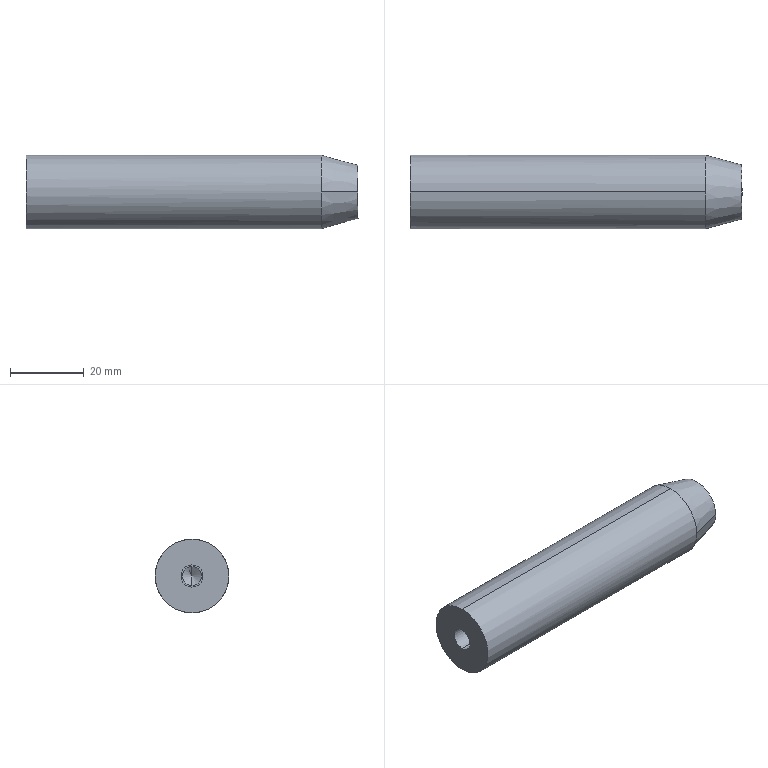Part | STEP file | [01]-15 | 1 solid | 13 faces | box 90 x 20 x 20 mm | volume 27097 mm3 | cylinder 6 | cone 4 | plane 3 | commonest cylinder face diameters 5.1 x2 6 x2 20 x2
STEP:
#1=CARTESIAN_POINT('',(0.,0.,0.));
#2=DIRECTION('',(0.,0.,1.));
#3=DIRECTION('',(1.,0.,0.));
#4=AXIS2_PLACEMENT_3D('',#1,#2,#3);
#5=CARTESIAN_POINT('',(15.,0.,-2.55));
#6=VERTEX_POINT('',#5);
#7=CARTESIAN_POINT('',(15.,0.,2.55));
#8=VERTEX_POINT('',#7);
#9=CARTESIAN_POINT('',(15.,0.,0.));
#10=DIRECTION('',(-1.,0.,0.));
#11=DIRECTION('',(0.,0.,1.));
#12=AXIS2_PLACEMENT_3D('',#9,#10,#11);
#13=CIRCLE('',#12,2.55);
#14=CARTESIAN_POINT('',(15.,0.,0.));
#15=DIRECTION('',(-1.,0.,0.));
#16=DIRECTION('',(0.,0.,1.));
#17=AXIS2_PLACEMENT_3D('',#14,#15,#16);
#18=CONICAL_SURFACE('',#17,2.55,1.03);
#19=CARTESIAN_POINT('',(0.,0.));
#20=DIRECTION('',(1.,0.));
#21=VECTOR('',#20,1.);
#22=LINE('',#19,#21);
#23=(GEOMETRIC_REPRESENTATION_CONTEXT(2)PARAMETRIC_REPRESENTATION_CONTEXT()REPRESENTATION_CONTEXT('',''));
#24=DEFINITIONAL_REPRESENTATION('',(#22),#23);
#25=PCURVE('',#18,#24);
#26=CARTESIAN_POINT('',(0.,0.,0.));
#27=DIRECTION('',(-1.,0.,0.));
#28=DIRECTION('',(0.,0.,1.));
#29=AXIS2_PLACEMENT_3D('',#26,#27,#28);
#30=CYLINDRICAL_SURFACE('',#29,2.55);
#31=CARTESIAN_POINT('',(0.,-15.));
#32=DIRECTION('',(1.,0.));
#33=VECTOR('',#32,1.);
#34=LINE('',#31,#33);
#35=(GEOMETRIC_REPRESENTATION_CONTEXT(2)PARAMETRIC_REPRESENTATION_CONTEXT()REPRESENTATION_CONTEXT('',''));
#36=DEFINITIONAL_REPRESENTATION('',(#34),#35);
#37=PCURVE('',#30,#36);
#38=SURFACE_CURVE('',#13,(#25,#37),.PCURVE_S1.);
#39=EDGE_CURVE('',#6,#8,#38,.T.);
#40=ORIENTED_EDGE('',*,*,#39,.F.);
#41=CARTESIAN_POINT('',(16.532,0.,0.));
#42=VERTEX_POINT('',#41);
#43=CARTESIAN_POINT('',(15.,0.,-2.55));
#44=DIRECTION('',(-0.515,0.,-0.8572));
#45=VECTOR('',#44,1.);
#46=LINE('',#43,#45);
#47=CARTESIAN_POINT('',(3.142,0.));
#48=DIRECTION('',(0.,1.));
#49=VECTOR('',#48,1.);
#50=LINE('',#47,#49);
#51=(GEOMETRIC_REPRESENTATION_CONTEXT(2)PARAMETRIC_REPRESENTATION_CONTEXT()REPRESENTATION_CONTEXT('',''));
#52=DEFINITIONAL_REPRESENTATION('',(#50),#51);
#53=PCURVE('',#18,#52);
#54=CARTESIAN_POINT('',(15.,0.,0.));
#55=DIRECTION('',(-1.,0.,0.));
#56=DIRECTION('',(0.,0.,1.));
#57=AXIS2_PLACEMENT_3D('',#54,#55,#56);
#58=CONICAL_SURFACE('',#57,2.55,1.03);
#59=CARTESIAN_POINT('',(3.142,0.));
#60=DIRECTION('',(0.,1.));
#61=VECTOR('',#60,1.);
#62=LINE('',#59,#61);
#63=(GEOMETRIC_REPRESENTATION_CONTEXT(2)PARAMETRIC_REPRESENTATION_CONTEXT()REPRESENTATION_CONTEXT('',''));
#64=DEFINITIONAL_REPRESENTATION('',(#62),#63);
#65=PCURVE('',#58,#64);
#66=SURFACE_CURVE('',#46,(#53,#65),.PCURVE_S1.);
#67=EDGE_CURVE('',#42,#6,#66,.T.);
#68=ORIENTED_EDGE('',*,*,#67,.F.);
#69=CARTESIAN_POINT('',(15.,0.,2.55));
#70=DIRECTION('',(-0.515,0.,0.8572));
#71=VECTOR('',#70,1.);
#72=LINE('',#69,#71);
#73=CARTESIAN_POINT('',(6.283,0.));
#74=DIRECTION('',(0.,1.));
#75=VECTOR('',#74,1.);
#76=LINE('',#73,#75);
#77=(GEOMETRIC_REPRESENTATION_CONTEXT(2)PARAMETRIC_REPRESENTATION_CONTEXT()REPRESENTATION_CONTEXT('',''));
#78=DEFINITIONAL_REPRESENTATION('',(#76),#77);
#79=PCURVE('',#18,#78);
#80=CARTESIAN_POINT('',(0.,0.));
#81=DIRECTION('',(0.,1.));
#82=VECTOR('',#81,1.);
#83=LINE('',#80,#82);
#84=(GEOMETRIC_REPRESENTATION_CONTEXT(2)PARAMETRIC_REPRESENTATION_CONTEXT()REPRESENTATION_CONTEXT('',''));
#85=DEFINITIONAL_REPRESENTATION('',(#83),#84);
#86=PCURVE('',#58,#85);
#87=SURFACE_CURVE('',#72,(#79,#86),.PCURVE_S1.);
#88=EDGE_CURVE('',#42,#8,#87,.T.);
#89=ORIENTED_EDGE('',*,*,#88,.T.);
#90=EDGE_LOOP('',(#40,#68,#89));
#91=FACE_BOUND('',#90,.F.);
#92=ADVANCED_FACE('',(#91),#18,.F.);
#93=CARTESIAN_POINT('',(12.,0.,2.55));
#94=VERTEX_POINT('',#93);
#95=CARTESIAN_POINT('',(0.,0.,2.55));
#96=DIRECTION('',(-1.,0.,0.));
#97=VECTOR('',#96,1.);
#98=LINE('',#95,#97);
#99=CARTESIAN_POINT('',(6.283,0.));
#100=DIRECTION('',(0.,1.));
#101=VECTOR('',#100,1.);
#102=LINE('',#99,#101);
#103=(GEOMETRIC_REPRESENTATION_CONTEXT(2)PARAMETRIC_REPRESENTATION_CONTEXT()REPRESENTATION_CONTEXT('',''));
#104=DEFINITIONAL_REPRESENTATION('',(#102),#103);
#105=PCURVE('',#30,#104);
#106=CARTESIAN_POINT('',(0.,0.,0.));
#107=DIRECTION('',(-1.,0.,0.));
#108=DIRECTION('',(0.,0.,1.));
#109=AXIS2_PLACEMENT_3D('',#106,#107,#108);
#110=CYLINDRICAL_SURFACE('',#109,2.55);
#111=CARTESIAN_POINT('',(0.,0.));
#112=DIRECTION('',(0.,1.));
#113=VECTOR('',#112,1.);
#114=LINE('',#111,#113);
#115=(GEOMETRIC_REPRESENTATION_CONTEXT(2)PARAMETRIC_REPRESENTATION_CONTEXT()REPRESENTATION_CONTEXT('',''));
#116=DEFINITIONAL_REPRESENTATION('',(#114),#115);
#117=PCURVE('',#110,#116);
#118=SURFACE_CURVE('',#98,(#105,#117),.PCURVE_S1.);
#119=EDGE_CURVE('',#8,#94,#118,.T.);
#120=ORIENTED_EDGE('',*,*,#119,.T.);
#121=CARTESIAN_POINT('',(12.,0.,-2.55));
#122=VERTEX_POINT('',#121);
#123=CARTESIAN_POINT('',(12.,0.,0.));
#124=DIRECTION('',(-1.,0.,0.));
#125=DIRECTION('',(0.,0.,1.));
#126=AXIS2_PLACEMENT_3D('',#123,#124,#125);
#127=CIRCLE('',#126,2.55);
#128=CARTESIAN_POINT('',(0.,-12.));
#129=DIRECTION('',(1.,0.));
#130=VECTOR('',#129,1.);
#131=LINE('',#128,#130);
#132=(GEOMETRIC_REPRESENTATION_CONTEXT(2)PARAMETRIC_REPRESENTATION_CONTEXT()REPRESENTATION_CONTEXT('',''));
#133=DEFINITIONAL_REPRESENTATION('',(#131),#132);
#134=PCURVE('',#30,#133);
#135=CARTESIAN_POINT('',(12.,0.,-3.));
#136=DIRECTION('',(1.,0.,0.));
#137=DIRECTION('',(0.,0.,-1.));
#138=AXIS2_PLACEMENT_3D('',#135,#136,#137);
#139=PLANE('',#138);
#140=CARTESIAN_POINT('',(-5.55,0.));
#141=CARTESIAN_POINT('',(-5.55,4.417));
#142=CARTESIAN_POINT('',(-1.725,2.208));
#143=CARTESIAN_POINT('',(2.1,0.));
#144=CARTESIAN_POINT('',(-1.725,-2.208));
#145=CARTESIAN_POINT('',(-5.55,-4.417));
#146=CARTESIAN_POINT('',(-5.55,0.));
#147=(BOUNDED_CURVE()B_SPLINE_CURVE(2,(#140,#141,#142,#143,#144,#145,#146),.UNSPECIFIED.,.T.,.F.)B_SPLINE_CURVE_WITH_KNOTS((1,2,2,2,2,1),(-2.094,0.,2.094,4.189,6.283,8.378),.UNSPECIFIED.)CURVE()GEOMETRIC_REPRESENTATION_ITEM()RATIONAL_B_SPLINE_CURVE((1.,0.5,1.,0.5,1.,0.5,1.))REPRESENTATION_ITEM(''));
#148=(GEOMETRIC_REPRESENTATION_CONTEXT(2)PARAMETRIC_REPRESENTATION_CONTEXT()REPRESENTATION_CONTEXT('',''));
#149=DEFINITIONAL_REPRESENTATION('',(#147),#148);
#150=PCURVE('',#139,#149);
#151=SURFACE_CURVE('',#127,(#134,#150),.PCURVE_S1.);
#152=EDGE_CURVE('',#122,#94,#151,.T.);
#153=ORIENTED_EDGE('',*,*,#152,.F.);
#154=CARTESIAN_POINT('',(0.,0.,-2.55));
#155=DIRECTION('',(-1.,0.,0.));
#156=VECTOR('',#155,1.);
#157=LINE('',#154,#156);
#158=CARTESIAN_POINT('',(3.142,0.));
#159=DIRECTION('',(0.,1.));
#160=VECTOR('',#159,1.);
#161=LINE('',#158,#160);
#162=(GEOMETRIC_REPRESENTATION_CONTEXT(2)PARAMETRIC_REPRESENTATION_CONTEXT()REPRESENTATION_CONTEXT('',''));
#163=DEFINITIONAL_REPRESENTATION('',(#161),#162);
#164=PCURVE('',#30,#163);
#165=CARTESIAN_POINT('',(3.142,0.));
#166=DIRECTION('',(0.,1.));
#167=VECTOR('',#166,1.);
#168=LINE('',#165,#167);
#169=(GEOMETRIC_REPRESENTATION_CONTEXT(2)PARAMETRIC_REPRESENTATION_CONTEXT()REPRESENTATION_CONTEXT('',''));
#170=DEFINITIONAL_REPRESENTATION('',(#168),#169);
#171=PCURVE('',#110,#170);
#172=SURFACE_CURVE('',#157,(#164,#171),.PCURVE_S1.);
#173=EDGE_CURVE('',#6,#122,#172,.T.);
#174=ORIENTED_EDGE('',*,*,#173,.F.);
#175=ORIENTED_EDGE('',*,*,#39,.T.);
#176=EDGE_LOOP('',(#120,#153,#174,#175));
#177=FACE_BOUND('',#176,.F.);
#178=ADVANCED_FACE('',(#177),#30,.F.);
#179=CARTESIAN_POINT('',(12.,0.,3.));
#180=VERTEX_POINT('',#179);
#181=CARTESIAN_POINT('',(0.,0.,3.));
#182=VERTEX_POINT('',#181);
#183=CARTESIAN_POINT('',(0.,0.,3.));
#184=DIRECTION('',(-1.,0.,0.));
#185=VECTOR('',#184,1.);
#186=LINE('',#183,#185);
#187=CARTESIAN_POINT('',(0.,0.,0.));
#188=DIRECTION('',(-1.,0.,0.));
#189=DIRECTION('',(0.,0.,1.));
#190=AXIS2_PLACEMENT_3D('',#187,#188,#189);
#191=CYLINDRICAL_SURFACE('',#190,3.);
#192=CARTESIAN_POINT('',(6.283,0.));
#193=DIRECTION('',(0.,1.));
#194=VECTOR('',#193,1.);
#195=LINE('',#192,#194);
#196=(GEOMETRIC_REPRESENTATION_CONTEXT(2)PARAMETRIC_REPRESENTATION_CONTEXT()REPRESENTATION_CONTEXT('',''));
#197=DEFINITIONAL_REPRESENTATION('',(#195),#196);
#198=PCURVE('',#191,#197);
#199=CARTESIAN_POINT('',(0.,0.,0.));
#200=DIRECTION('',(-1.,0.,0.));
#201=DIRECTION('',(0.,0.,1.));
#202=AXIS2_PLACEMENT_3D('',#199,#200,#201);
#203=CYLINDRICAL_SURFACE('',#202,3.);
#204=CARTESIAN_POINT('',(0.,0.));
#205=DIRECTION('',(0.,1.));
#206=VECTOR('',#205,1.);
#207=LINE('',#204,#206);
#208=(GEOMETRIC_REPRESENTATION_CONTEXT(2)PARAMETRIC_REPRESENTATION_CONTEXT()REPRESENTATION_CONTEXT('',''));
#209=DEFINITIONAL_REPRESENTATION('',(#207),#208);
#210=PCURVE('',#203,#209);
#211=SURFACE_CURVE('',#186,(#198,#210),.PCURVE_S1.);
#212=EDGE_CURVE('',#180,#182,#211,.T.);
#213=ORIENTED_EDGE('',*,*,#212,.T.);
#214=CARTESIAN_POINT('',(0.,0.,-3.));
#215=VERTEX_POINT('',#214);
#216=CARTESIAN_POINT('',(0.,0.,0.));
#217=DIRECTION('',(-1.,0.,0.));
#218=DIRECTION('',(0.,0.,1.));
#219=AXIS2_PLACEMENT_3D('',#216,#217,#218);
#220=CIRCLE('',#219,3.);
#221=CARTESIAN_POINT('',(0.,0.));
#222=DIRECTION('',(1.,0.));
#223=VECTOR('',#222,1.);
#224=LINE('',#221,#223);
#225=(GEOMETRIC_REPRESENTATION_CONTEXT(2)PARAMETRIC_REPRESENTATION_CONTEXT()REPRESENTATION_CONTEXT('',''));
#226=DEFINITIONAL_REPRESENTATION('',(#224),#225);
#227=PCURVE('',#191,#226);
#228=CARTESIAN_POINT('',(0.,0.,0.));
#229=DIRECTION('',(-1.,0.,0.));
#230=DIRECTION('',(0.,0.,1.));
#231=AXIS2_PLACEMENT_3D('',#228,#229,#230);
#232=PLANE('',#231);
#233=CARTESIAN_POINT('',(0.,0.));
#234=DIRECTION('',(1.,0.));
#235=AXIS2_PLACEMENT_2D('',#233,#234);
#236=CIRCLE('',#235,3.);
#237=(GEOMETRIC_REPRESENTATION_CONTEXT(2)PARAMETRIC_REPRESENTATION_CONTEXT()REPRESENTATION_CONTEXT('',''));
#238=DEFINITIONAL_REPRESENTATION('',(#236),#237);
#239=PCURVE('',#232,#238);
#240=SURFACE_CURVE('',#220,(#227,#239),.PCURVE_S1.);
#241=EDGE_CURVE('',#215,#182,#240,.T.);
#242=ORIENTED_EDGE('',*,*,#241,.F.);
#243=CARTESIAN_POINT('',(12.,0.,-3.));
#244=VERTEX_POINT('',#243);
#245=CARTESIAN_POINT('',(0.,0.,-3.));
#246=DIRECTION('',(-1.,0.,0.));
#247=VECTOR('',#246,1.);
#248=LINE('',#245,#247);
#249=CARTESIAN_POINT('',(3.142,0.));
#250=DIRECTION('',(0.,1.));
#251=VECTOR('',#250,1.);
#252=LINE('',#249,#251);
#253=(GEOMETRIC_REPRESENTATION_CONTEXT(2)PARAMETRIC_REPRESENTATION_CONTEXT()REPRESENTATION_CONTEXT('',''));
#254=DEFINITIONAL_REPRESENTATION('',(#252),#253);
#255=PCURVE('',#191,#254);
#256=CARTESIAN_POINT('',(3.142,0.));
#257=DIRECTION('',(0.,1.));
#258=VECTOR('',#257,1.);
#259=LINE('',#256,#258);
#260=(GEOMETRIC_REPRESENTATION_CONTEXT(2)PARAMETRIC_REPRESENTATION_CONTEXT()REPRESENTATION_CONTEXT('',''));
#261=DEFINITIONAL_REPRESENTATION('',(#259),#260);
#262=PCURVE('',#203,#261);
#263=SURFACE_CURVE('',#248,(#255,#262),.PCURVE_S1.);
#264=EDGE_CURVE('',#244,#215,#263,.T.);
#265=ORIENTED_EDGE('',*,*,#264,.F.);
#266=CARTESIAN_POINT('',(12.,0.,0.));
#267=DIRECTION('',(-1.,0.,0.));
#268=DIRECTION('',(0.,0.,1.));
#269=AXIS2_PLACEMENT_3D('',#266,#267,#268);
#270=CIRCLE('',#269,3.);
#271=CARTESIAN_POINT('',(0.,-12.));
#272=DIRECTION('',(1.,0.));
#273=VECTOR('',#272,1.);
#274=LINE('',#271,#273);
#275=(GEOMETRIC_REPRESENTATION_CONTEXT(2)PARAMETRIC_REPRESENTATION_CONTEXT()REPRESENTATION_CONTEXT('',''));
#276=DEFINITIONAL_REPRESENTATION('',(#274),#275);
#277=PCURVE('',#191,#276);
#278=CARTESIAN_POINT('',(-6.,0.));
#279=CARTESIAN_POINT('',(-6.,5.196));
#280=CARTESIAN_POINT('',(-1.5,2.598));
#281=CARTESIAN_POINT('',(3.,0.));
#282=CARTESIAN_POINT('',(-1.5,-2.598));
#283=CARTESIAN_POINT('',(-6.,-5.196));
#284=CARTESIAN_POINT('',(-6.,0.));
#285=(BOUNDED_CURVE()B_SPLINE_CURVE(2,(#278,#279,#280,#281,#282,#283,#284),.UNSPECIFIED.,.T.,.F.)B_SPLINE_CURVE_WITH_KNOTS((1,2,2,2,2,1),(-2.094,0.,2.094,4.189,6.283,8.378),.UNSPECIFIED.)CURVE()GEOMETRIC_REPRESENTATION_ITEM()RATIONAL_B_SPLINE_CURVE((1.,0.5,1.,0.5,1.,0.5,1.))REPRESENTATION_ITEM(''));
#286=(GEOMETRIC_REPRESENTATION_CONTEXT(2)PARAMETRIC_REPRESENTATION_CONTEXT()REPRESENTATION_CONTEXT('',''));
#287=DEFINITIONAL_REPRESENTATION('',(#285),#286);
#288=PCURVE('',#139,#287);
#289=SURFACE_CURVE('',#270,(#277,#288),.PCURVE_S1.);
#290=EDGE_CURVE('',#244,#180,#289,.T.);
#291=ORIENTED_EDGE('',*,*,#290,.T.);
#292=EDGE_LOOP('',(#213,#242,#265,#291));
#293=FACE_BOUND('',#292,.F.);
#294=ADVANCED_FACE('',(#293),#191,.F.);
#295=CARTESIAN_POINT('',(0.,0.,-10.));
#296=VERTEX_POINT('',#295);
#297=CARTESIAN_POINT('',(0.,0.,10.));
#298=VERTEX_POINT('',#297);
#299=CARTESIAN_POINT('',(0.,0.,0.));
#300=DIRECTION('',(1.,0.,0.));
#301=DIRECTION('',(0.,0.,-1.));
#302=AXIS2_PLACEMENT_3D('',#299,#300,#301);
#303=CIRCLE('',#302,10.);
#304=CARTESIAN_POINT('',(0.,0.,0.));
#305=DIRECTION('',(1.,0.,0.));
#306=DIRECTION('',(0.,0.,-1.));
#307=AXIS2_PLACEMENT_3D('',#304,#305,#306);
#308=CYLINDRICAL_SURFACE('',#307,10.);
#309=CARTESIAN_POINT('',(0.,0.));
#310=DIRECTION('',(1.,0.));
#311=VECTOR('',#310,1.);
#312=LINE('',#309,#311);
#313=(GEOMETRIC_REPRESENTATION_CONTEXT(2)PARAMETRIC_REPRESENTATION_CONTEXT()REPRESENTATION_CONTEXT('',''));
#314=DEFINITIONAL_REPRESENTATION('',(#312),#313);
#315=PCURVE('',#308,#314);
#316=CARTESIAN_POINT('',(-10.,0.));
#317=CARTESIAN_POINT('',(-10.,17.321));
#318=CARTESIAN_POINT('',(5.,8.66));
#319=CARTESIAN_POINT('',(20.,0.));
#320=CARTESIAN_POINT('',(5.,-8.66));
#321=CARTESIAN_POINT('',(-10.,-17.321));
#322=CARTESIAN_POINT('',(-10.,0.));
#323=(BOUNDED_CURVE()B_SPLINE_CURVE(2,(#316,#317,#318,#319,#320,#321,#322),.UNSPECIFIED.,.T.,.F.)B_SPLINE_CURVE_WITH_KNOTS((1,2,2,2,2,1),(-2.094,0.,2.094,4.189,6.283,8.378),.UNSPECIFIED.)CURVE()GEOMETRIC_REPRESENTATION_ITEM()RATIONAL_B_SPLINE_CURVE((1.,0.5,1.,0.5,1.,0.5,1.))REPRESENTATION_ITEM(''));
#324=(GEOMETRIC_REPRESENTATION_CONTEXT(2)PARAMETRIC_REPRESENTATION_CONTEXT()REPRESENTATION_CONTEXT('',''));
#325=DEFINITIONAL_REPRESENTATION('',(#323),#324);
#326=PCURVE('',#232,#325);
#327=SURFACE_CURVE('',#303,(#315,#326),.PCURVE_S1.);
#328=EDGE_CURVE('',#296,#298,#327,.T.);
#329=ORIENTED_EDGE('',*,*,#328,.T.);
#330=CARTESIAN_POINT('',(80.,0.,10.));
#331=VERTEX_POINT('',#330);
#332=CARTESIAN_POINT('',(0.,0.,10.));
#333=DIRECTION('',(1.,0.,0.));
#334=VECTOR('',#333,1.);
#335=LINE('',#332,#334);
#336=CARTESIAN_POINT('',(3.142,0.));
#337=DIRECTION('',(0.,1.));
#338=VECTOR('',#337,1.);
#339=LINE('',#336,#338);
#340=(GEOMETRIC_REPRESENTATION_CONTEXT(2)PARAMETRIC_REPRESENTATION_CONTEXT()REPRESENTATION_CONTEXT('',''));
#341=DEFINITIONAL_REPRESENTATION('',(#339),#340);
#342=PCURVE('',#308,#341);
#343=CARTESIAN_POINT('',(0.,0.,0.));
#344=DIRECTION('',(1.,0.,0.));
#345=DIRECTION('',(0.,0.,-1.));
#346=AXIS2_PLACEMENT_3D('',#343,#344,#345);
#347=CYLINDRICAL_SURFACE('',#346,10.);
#348=CARTESIAN_POINT('',(3.142,0.));
#349=DIRECTION('',(0.,1.));
#350=VECTOR('',#349,1.);
#351=LINE('',#348,#350);
#352=(GEOMETRIC_REPRESENTATION_CONTEXT(2)PARAMETRIC_REPRESENTATION_CONTEXT()REPRESENTATION_CONTEXT('',''));
#353=DEFINITIONAL_REPRESENTATION('',(#351),#352);
#354=PCURVE('',#347,#353);
#355=SURFACE_CURVE('',#335,(#342,#354),.PCURVE_S1.);
#356=EDGE_CURVE('',#298,#331,#355,.T.);
#357=ORIENTED_EDGE('',*,*,#356,.T.);
#358=CARTESIAN_POINT('',(80.,10.,0.));
#359=VERTEX_POINT('',#358);
#360=CARTESIAN_POINT('',(80.,0.,0.));
#361=DIRECTION('',(-1.,0.,0.));
#362=DIRECTION('',(0.,0.,1.));
#363=AXIS2_PLACEMENT_3D('',#360,#361,#362);
#364=CIRCLE('',#363,10.);
#365=CARTESIAN_POINT('',(3.142,80.));
#366=DIRECTION('',(-1.,0.));
#367=VECTOR('',#366,1.);
#368=LINE('',#365,#367);
#369=(GEOMETRIC_REPRESENTATION_CONTEXT(2)PARAMETRIC_REPRESENTATION_CONTEXT()REPRESENTATION_CONTEXT('',''));
#370=DEFINITIONAL_REPRESENTATION('',(#368),#369);
#371=PCURVE('',#308,#370);
#372=CARTESIAN_POINT('',(90.,0.,0.));
#373=DIRECTION('',(-1.,0.,0.));
#374=DIRECTION('',(0.,1.,0.));
#375=AXIS2_PLACEMENT_3D('',#372,#373,#374);
#376=CONICAL_SURFACE('',#375,7.321,0.2618);
#377=CARTESIAN_POINT('',(4.712,10.));
#378=DIRECTION('',(1.,0.));
#379=VECTOR('',#378,1.);
#380=LINE('',#377,#379);
#381=(GEOMETRIC_REPRESENTATION_CONTEXT(2)PARAMETRIC_REPRESENTATION_CONTEXT()REPRESENTATION_CONTEXT('',''));
#382=DEFINITIONAL_REPRESENTATION('',(#380),#381);
#383=PCURVE('',#376,#382);
#384=SURFACE_CURVE('',#364,(#371,#383),.PCURVE_S1.);
#385=EDGE_CURVE('',#331,#359,#384,.T.);
#386=ORIENTED_EDGE('',*,*,#385,.T.);
#387=CARTESIAN_POINT('',(80.,0.,-10.));
#388=VERTEX_POINT('',#387);
#389=CARTESIAN_POINT('',(80.,0.,0.));
#390=DIRECTION('',(-1.,0.,0.));
#391=DIRECTION('',(0.,0.,1.));
#392=AXIS2_PLACEMENT_3D('',#389,#390,#391);
#393=CIRCLE('',#392,10.);
#394=CARTESIAN_POINT('',(3.142,80.));
#395=DIRECTION('',(-1.,0.));
#396=VECTOR('',#395,1.);
#397=LINE('',#394,#396);
#398=(GEOMETRIC_REPRESENTATION_CONTEXT(2)PARAMETRIC_REPRESENTATION_CONTEXT()REPRESENTATION_CONTEXT('',''));
#399=DEFINITIONAL_REPRESENTATION('',(#397),#398);
#400=PCURVE('',#308,#399);
#401=CARTESIAN_POINT('',(90.,0.,0.));
#402=DIRECTION('',(-1.,0.,0.));
#403=DIRECTION('',(0.,1.,0.));
#404=AXIS2_PLACEMENT_3D('',#401,#402,#403);
#405=CONICAL_SURFACE('',#404,7.321,0.2618);
#406=CARTESIAN_POINT('',(-1.571,10.));
#407=DIRECTION('',(1.,0.));
#408=VECTOR('',#407,1.);
#409=LINE('',#406,#408);
#410=(GEOMETRIC_REPRESENTATION_CONTEXT(2)PARAMETRIC_REPRESENTATION_CONTEXT()REPRESENTATION_CONTEXT('',''));
#411=DEFINITIONAL_REPRESENTATION('',(#409),#410);
#412=PCURVE('',#405,#411);
#413=SURFACE_CURVE('',#393,(#400,#412),.PCURVE_S1.);
#414=EDGE_CURVE('',#359,#388,#413,.T.);
#415=ORIENTED_EDGE('',*,*,#414,.T.);
#416=CARTESIAN_POINT('',(0.,0.,-10.));
#417=DIRECTION('',(1.,0.,0.));
#418=VECTOR('',#417,1.);
#419=LINE('',#416,#418);
#420=CARTESIAN_POINT('',(0.,0.));
#421=DIRECTION('',(0.,1.));
#422=VECTOR('',#421,1.);
#423=LINE('',#420,#422);
#424=(GEOMETRIC_REPRESENTATION_CONTEXT(2)PARAMETRIC_REPRESENTATION_CONTEXT()REPRESENTATION_CONTEXT('',''));
#425=DEFINITIONAL_REPRESENTATION('',(#423),#424);
#426=PCURVE('',#308,#425);
#427=CARTESIAN_POINT('',(6.283,0.));
#428=DIRECTION('',(0.,1.));
#429=VECTOR('',#428,1.);
#430=LINE('',#427,#429);
#431=(GEOMETRIC_REPRESENTATION_CONTEXT(2)PARAMETRIC_REPRESENTATION_CONTEXT()REPRESENTATION_CONTEXT('',''));
#432=DEFINITIONAL_REPRESENTATION('',(#430),#431);
#433=PCURVE('',#347,#432);
#434=SURFACE_CURVE('',#419,(#426,#433),.PCURVE_S1.);
#435=EDGE_CURVE('',#296,#388,#434,.T.);
#436=ORIENTED_EDGE('',*,*,#435,.F.);
#437=EDGE_LOOP('',(#329,#357,#386,#415,#436));
#438=FACE_BOUND('',#437,.T.);
#439=ADVANCED_FACE('',(#438),#308,.T.);
#440=CARTESIAN_POINT('',(90.,7.321,0.));
#441=VERTEX_POINT('',#440);
#442=CARTESIAN_POINT('',(90.,-7.321,0.));
#443=VERTEX_POINT('',#442);
#444=CARTESIAN_POINT('',(90.,0.,0.));
#445=DIRECTION('',(-1.,0.,0.));
#446=DIRECTION('',(0.,1.,0.));
#447=AXIS2_PLACEMENT_3D('',#444,#445,#446);
#448=CIRCLE('',#447,7.321);
#449=CARTESIAN_POINT('',(0.,0.));
#450=DIRECTION('',(1.,0.));
#451=VECTOR('',#450,1.);
#452=LINE('',#449,#451);
#453=(GEOMETRIC_REPRESENTATION_CONTEXT(2)PARAMETRIC_REPRESENTATION_CONTEXT()REPRESENTATION_CONTEXT('',''));
#454=DEFINITIONAL_REPRESENTATION('',(#452),#453);
#455=PCURVE('',#405,#454);
#456=CARTESIAN_POINT('',(90.,0.,0.));
#457=DIRECTION('',(1.,0.,0.));
#458=DIRECTION('',(0.,-1.,0.));
#459=AXIS2_PLACEMENT_3D('',#456,#457,#458);
#460=PLANE('',#459);
#461=CARTESIAN_POINT('',(-7.321,0.));
#462=CARTESIAN_POINT('',(-7.321,12.679));
#463=CARTESIAN_POINT('',(3.66,6.34));
#464=CARTESIAN_POINT('',(14.641,0.));
#465=CARTESIAN_POINT('',(3.66,-6.34));
#466=CARTESIAN_POINT('',(-7.321,-12.679));
#467=CARTESIAN_POINT('',(-7.321,0.));
#468=(BOUNDED_CURVE()B_SPLINE_CURVE(2,(#461,#462,#463,#464,#465,#466,#467),.UNSPECIFIED.,.T.,.F.)B_SPLINE_CURVE_WITH_KNOTS((1,2,2,2,2,1),(-2.094,0.,2.094,4.189,6.283,8.378),.UNSPECIFIED.)CURVE()GEOMETRIC_REPRESENTATION_ITEM()RATIONAL_B_SPLINE_CURVE((1.,0.5,1.,0.5,1.,0.5,1.))REPRESENTATION_ITEM(''));
#469=(GEOMETRIC_REPRESENTATION_CONTEXT(2)PARAMETRIC_REPRESENTATION_CONTEXT()REPRESENTATION_CONTEXT('',''));
#470=DEFINITIONAL_REPRESENTATION('',(#468),#469);
#471=PCURVE('',#460,#470);
#472=SURFACE_CURVE('',#448,(#455,#471),.PCURVE_S1.);
#473=EDGE_CURVE('',#441,#443,#472,.T.);
#474=ORIENTED_EDGE('',*,*,#473,.T.);
#475=CARTESIAN_POINT('',(80.,-10.,0.));
#476=VERTEX_POINT('',#475);
#477=CARTESIAN_POINT('',(90.,-7.321,0.));
#478=DIRECTION('',(-0.9659,-0.2588,0.));
#479=VECTOR('',#478,1.);
#480=LINE('',#477,#479);
#481=CARTESIAN_POINT('',(3.142,0.));
#482=DIRECTION('',(0.,1.));
#483=VECTOR('',#482,1.);
#484=LINE('',#481,#483);
#485=(GEOMETRIC_REPRESENTATION_CONTEXT(2)PARAMETRIC_REPRESENTATION_CONTEXT()REPRESENTATION_CONTEXT('',''));
#486=DEFINITIONAL_REPRESENTATION('',(#484),#485);
#487=PCURVE('',#405,#486);
#488=CARTESIAN_POINT('',(3.142,0.));
#489=DIRECTION('',(0.,1.));
#490=VECTOR('',#489,1.);
#491=LINE('',#488,#490);
#492=(GEOMETRIC_REPRESENTATION_CONTEXT(2)PARAMETRIC_REPRESENTATION_CONTEXT()REPRESENTATION_CONTEXT('',''));
#493=DEFINITIONAL_REPRESENTATION('',(#491),#492);
#494=PCURVE('',#376,#493);
#495=SURFACE_CURVE('',#480,(#487,#494),.PCURVE_S1.);
#496=EDGE_CURVE('',#443,#476,#495,.T.);
#497=ORIENTED_EDGE('',*,*,#496,.T.);
#498=CARTESIAN_POINT('',(80.,0.,0.));
#499=DIRECTION('',(-1.,0.,0.));
#500=DIRECTION('',(0.,0.,1.));
#501=AXIS2_PLACEMENT_3D('',#498,#499,#500);
#502=CIRCLE('',#501,10.);
#503=CARTESIAN_POINT('',(-1.571,10.));
#504=DIRECTION('',(1.,0.));
#505=VECTOR('',#504,1.);
#506=LINE('',#503,#505);
#507=(GEOMETRIC_REPRESENTATION_CONTEXT(2)PARAMETRIC_REPRESENTATION_CONTEXT()REPRESENTATION_CONTEXT('',''));
#508=DEFINITIONAL_REPRESENTATION('',(#506),#507);
#509=PCURVE('',#405,#508);
#510=CARTESIAN_POINT('',(9.425,80.));
#511=DIRECTION('',(-1.,0.));
#512=VECTOR('',#511,1.);
#513=LINE('',#510,#512);
#514=(GEOMETRIC_REPRESENTATION_CONTEXT(2)PARAMETRIC_REPRESENTATION_CONTEXT()REPRESENTATION_CONTEXT('',''));
#515=DEFINITIONAL_REPRESENTATION('',(#513),#514);
#516=PCURVE('',#347,#515);
#517=SURFACE_CURVE('',#502,(#509,#516),.PCURVE_S1.);
#518=EDGE_CURVE('',#388,#476,#517,.T.);
#519=ORIENTED_EDGE('',*,*,#518,.F.);
#520=ORIENTED_EDGE('',*,*,#414,.F.);
#521=CARTESIAN_POINT('',(90.,7.321,0.));
#522=DIRECTION('',(-0.9659,0.2588,0.));
#523=VECTOR('',#522,1.);
#524=LINE('',#521,#523);
#525=CARTESIAN_POINT('',(0.,0.));
#526=DIRECTION('',(0.,1.));
#527=VECTOR('',#526,1.);
#528=LINE('',#525,#527);
#529=(GEOMETRIC_REPRESENTATION_CONTEXT(2)PARAMETRIC_REPRESENTATION_CONTEXT()REPRESENTATION_CONTEXT('',''));
#530=DEFINITIONAL_REPRESENTATION('',(#528),#529);
#531=PCURVE('',#405,#530);
#532=CARTESIAN_POINT('',(6.283,0.));
#533=DIRECTION('',(0.,1.));
#534=VECTOR('',#533,1.);
#535=LINE('',#532,#534);
#536=(GEOMETRIC_REPRESENTATION_CONTEXT(2)PARAMETRIC_REPRESENTATION_CONTEXT()REPRESENTATION_CONTEXT('',''));
#537=DEFINITIONAL_REPRESENTATION('',(#535),#536);
#538=PCURVE('',#376,#537);
#539=SURFACE_CURVE('',#524,(#531,#538),.PCURVE_S1.);
#540=EDGE_CURVE('',#441,#359,#539,.T.);
#541=ORIENTED_EDGE('',*,*,#540,.F.);
#542=EDGE_LOOP('',(#474,#497,#519,#520,#541));
#543=FACE_BOUND('',#542,.T.);
#544=ADVANCED_FACE('',(#543),#405,.T.);
#545=ORIENTED_EDGE('',*,*,#473,.F.);
#546=CARTESIAN_POINT('',(90.,0.,0.));
#547=DIRECTION('',(-1.,0.,0.));
#548=DIRECTION('',(0.,1.,0.));
#549=AXIS2_PLACEMENT_3D('',#546,#547,#548);
#550=CIRCLE('',#549,7.321);
#551=CARTESIAN_POINT('',(-7.321,0.));
#552=CARTESIAN_POINT('',(-7.321,12.679));
#553=CARTESIAN_POINT('',(3.66,6.34));
#554=CARTESIAN_POINT('',(14.641,0.));
#555=CARTESIAN_POINT('',(3.66,-6.34));
#556=CARTESIAN_POINT('',(-7.321,-12.679));
#557=CARTESIAN_POINT('',(-7.321,0.));
#558=(BOUNDED_CURVE()B_SPLINE_CURVE(2,(#551,#552,#553,#554,#555,#556,#557),.UNSPECIFIED.,.T.,.F.)B_SPLINE_CURVE_WITH_KNOTS((1,2,2,2,2,1),(-2.094,0.,2.094,4.189,6.283,8.378),.UNSPECIFIED.)CURVE()GEOMETRIC_REPRESENTATION_ITEM()RATIONAL_B_SPLINE_CURVE((1.,0.5,1.,0.5,1.,0.5,1.))REPRESENTATION_ITEM(''));
#559=(GEOMETRIC_REPRESENTATION_CONTEXT(2)PARAMETRIC_REPRESENTATION_CONTEXT()REPRESENTATION_CONTEXT('',''));
#560=DEFINITIONAL_REPRESENTATION('',(#558),#559);
#561=PCURVE('',#460,#560);
#562=CARTESIAN_POINT('',(0.,0.));
#563=DIRECTION('',(1.,0.));
#564=VECTOR('',#563,1.);
#565=LINE('',#562,#564);
#566=(GEOMETRIC_REPRESENTATION_CONTEXT(2)PARAMETRIC_REPRESENTATION_CONTEXT()REPRESENTATION_CONTEXT('',''));
#567=DEFINITIONAL_REPRESENTATION('',(#565),#566);
#568=PCURVE('',#376,#567);
#569=SURFACE_CURVE('',#550,(#561,#568),.PCURVE_S1.);
#570=EDGE_CURVE('',#443,#441,#569,.T.);
#571=ORIENTED_EDGE('',*,*,#570,.F.);
#572=EDGE_LOOP('',(#545,#571));
#573=FACE_BOUND('',#572,.T.);
#574=ADVANCED_FACE('',(#573),#460,.T.);
#575=ORIENTED_EDGE('',*,*,#496,.F.);
#576=ORIENTED_EDGE('',*,*,#570,.T.);
#577=ORIENTED_EDGE('',*,*,#540,.T.);
#578=ORIENTED_EDGE('',*,*,#385,.F.);
#579=CARTESIAN_POINT('',(80.,0.,0.));
#580=DIRECTION('',(-1.,0.,0.));
#581=DIRECTION('',(0.,0.,1.));
#582=AXIS2_PLACEMENT_3D('',#579,#580,#581);
#583=CIRCLE('',#582,10.);
#584=CARTESIAN_POINT('',(-1.571,10.));
#585=DIRECTION('',(1.,0.));
#586=VECTOR('',#585,1.);
#587=LINE('',#584,#586);
#588=(GEOMETRIC_REPRESENTATION_CONTEXT(2)PARAMETRIC_REPRESENTATION_CONTEXT()REPRESENTATION_CONTEXT('',''));
#589=DEFINITIONAL_REPRESENTATION('',(#587),#588);
#590=PCURVE('',#376,#589);
#591=CARTESIAN_POINT('',(9.425,80.));
#592=DIRECTION('',(-1.,0.));
#593=VECTOR('',#592,1.);
#594=LINE('',#591,#593);
#595=(GEOMETRIC_REPRESENTATION_CONTEXT(2)PARAMETRIC_REPRESENTATION_CONTEXT()REPRESENTATION_CONTEXT('',''));
#596=DEFINITIONAL_REPRESENTATION('',(#594),#595);
#597=PCURVE('',#347,#596);
#598=SURFACE_CURVE('',#583,(#590,#597),.PCURVE_S1.);
#599=EDGE_CURVE('',#476,#331,#598,.T.);
#600=ORIENTED_EDGE('',*,*,#599,.F.);
#601=EDGE_LOOP('',(#575,#576,#577,#578,#600));
#602=FACE_BOUND('',#601,.T.);
#603=ADVANCED_FACE('',(#602),#376,.T.);
#604=CARTESIAN_POINT('',(0.,0.,0.));
#605=DIRECTION('',(-1.,0.,0.));
#606=DIRECTION('',(0.,0.,1.));
#607=AXIS2_PLACEMENT_3D('',#604,#605,#606);
#608=CIRCLE('',#607,3.);
#609=CARTESIAN_POINT('',(0.,0.));
#610=DIRECTION('',(1.,0.));
#611=AXIS2_PLACEMENT_2D('',#609,#610);
#612=CIRCLE('',#611,3.);
#613=(GEOMETRIC_REPRESENTATION_CONTEXT(2)PARAMETRIC_REPRESENTATION_CONTEXT()REPRESENTATION_CONTEXT('',''));
#614=DEFINITIONAL_REPRESENTATION('',(#612),#613);
#615=PCURVE('',#232,#614);
#616=CARTESIAN_POINT('',(0.,0.));
#617=DIRECTION('',(1.,0.));
#618=VECTOR('',#617,1.);
#619=LINE('',#616,#618);
#620=(GEOMETRIC_REPRESENTATION_CONTEXT(2)PARAMETRIC_REPRESENTATION_CONTEXT()REPRESENTATION_CONTEXT('',''));
#621=DEFINITIONAL_REPRESENTATION('',(#619),#620);
#622=PCURVE('',#203,#621);
#623=SURFACE_CURVE('',#608,(#615,#622),.PCURVE_S1.);
#624=EDGE_CURVE('',#182,#215,#623,.T.);
#625=ORIENTED_EDGE('',*,*,#624,.F.);
#626=ORIENTED_EDGE('',*,*,#241,.F.);
#627=EDGE_LOOP('',(#625,#626));
#628=FACE_BOUND('',#627,.T.);
#629=ORIENTED_EDGE('',*,*,#328,.F.);
#630=CARTESIAN_POINT('',(0.,0.,0.));
#631=DIRECTION('',(1.,0.,0.));
#632=DIRECTION('',(0.,0.,-1.));
#633=AXIS2_PLACEMENT_3D('',#630,#631,#632);
#634=CIRCLE('',#633,10.);
#635=CARTESIAN_POINT('',(-10.,0.));
#636=CARTESIAN_POINT('',(-10.,17.321));
#637=CARTESIAN_POINT('',(5.,8.66));
#638=CARTESIAN_POINT('',(20.,0.));
#639=CARTESIAN_POINT('',(5.,-8.66));
#640=CARTESIAN_POINT('',(-10.,-17.321));
#641=CARTESIAN_POINT('',(-10.,0.));
#642=(BOUNDED_CURVE()B_SPLINE_CURVE(2,(#635,#636,#637,#638,#639,#640,#641),.UNSPECIFIED.,.T.,.F.)B_SPLINE_CURVE_WITH_KNOTS((1,2,2,2,2,1),(-2.094,0.,2.094,4.189,6.283,8.378),.UNSPECIFIED.)CURVE()GEOMETRIC_REPRESENTATION_ITEM()RATIONAL_B_SPLINE_CURVE((1.,0.5,1.,0.5,1.,0.5,1.))REPRESENTATION_ITEM(''));
#643=(GEOMETRIC_REPRESENTATION_CONTEXT(2)PARAMETRIC_REPRESENTATION_CONTEXT()REPRESENTATION_CONTEXT('',''));
#644=DEFINITIONAL_REPRESENTATION('',(#642),#643);
#645=PCURVE('',#232,#644);
#646=CARTESIAN_POINT('',(0.,0.));
#647=DIRECTION('',(1.,0.));
#648=VECTOR('',#647,1.);
#649=LINE('',#646,#648);
#650=(GEOMETRIC_REPRESENTATION_CONTEXT(2)PARAMETRIC_REPRESENTATION_CONTEXT()REPRESENTATION_CONTEXT('',''));
#651=DEFINITIONAL_REPRESENTATION('',(#649),#650);
#652=PCURVE('',#347,#651);
#653=SURFACE_CURVE('',#634,(#645,#652),.PCURVE_S1.);
#654=EDGE_CURVE('',#298,#296,#653,.T.);
#655=ORIENTED_EDGE('',*,*,#654,.F.);
#656=EDGE_LOOP('',(#629,#655));
#657=FACE_BOUND('',#656,.T.);
#658=ADVANCED_FACE('',(#628,#657),#232,.T.);
#659=ORIENTED_EDGE('',*,*,#356,.F.);
#660=ORIENTED_EDGE('',*,*,#654,.T.);
#661=ORIENTED_EDGE('',*,*,#435,.T.);
#662=ORIENTED_EDGE('',*,*,#518,.T.);
#663=ORIENTED_EDGE('',*,*,#599,.T.);
#664=EDGE_LOOP('',(#659,#660,#661,#662,#663));
#665=FACE_BOUND('',#664,.T.);
#666=ADVANCED_FACE('',(#665),#347,.T.);
#667=ORIENTED_EDGE('',*,*,#624,.F.);
#668=ORIENTED_EDGE('',*,*,#212,.F.);
#669=CARTESIAN_POINT('',(12.,0.,0.));
#670=DIRECTION('',(-1.,0.,0.));
#671=DIRECTION('',(0.,0.,1.));
#672=AXIS2_PLACEMENT_3D('',#669,#670,#671);
#673=CIRCLE('',#672,3.);
#674=CARTESIAN_POINT('',(0.,-12.));
#675=DIRECTION('',(1.,0.));
#676=VECTOR('',#675,1.);
#677=LINE('',#674,#676);
#678=(GEOMETRIC_REPRESENTATION_CONTEXT(2)PARAMETRIC_REPRESENTATION_CONTEXT()REPRESENTATION_CONTEXT('',''));
#679=DEFINITIONAL_REPRESENTATION('',(#677),#678);
#680=PCURVE('',#203,#679);
#681=CARTESIAN_POINT('',(-6.,0.));
#682=CARTESIAN_POINT('',(-6.,5.196));
#683=CARTESIAN_POINT('',(-1.5,2.598));
#684=CARTESIAN_POINT('',(3.,0.));
#685=CARTESIAN_POINT('',(-1.5,-2.598));
#686=CARTESIAN_POINT('',(-6.,-5.196));
#687=CARTESIAN_POINT('',(-6.,0.));
#688=(BOUNDED_CURVE()B_SPLINE_CURVE(2,(#681,#682,#683,#684,#685,#686,#687),.UNSPECIFIED.,.T.,.F.)B_SPLINE_CURVE_WITH_KNOTS((1,2,2,2,2,1),(-2.094,0.,2.094,4.189,6.283,8.378),.UNSPECIFIED.)CURVE()GEOMETRIC_REPRESENTATION_ITEM()RATIONAL_B_SPLINE_CURVE((1.,0.5,1.,0.5,1.,0.5,1.))REPRESENTATION_ITEM(''));
#689=(GEOMETRIC_REPRESENTATION_CONTEXT(2)PARAMETRIC_REPRESENTATION_CONTEXT()REPRESENTATION_CONTEXT('',''));
#690=DEFINITIONAL_REPRESENTATION('',(#688),#689);
#691=PCURVE('',#139,#690);
#692=SURFACE_CURVE('',#673,(#680,#691),.PCURVE_S1.);
#693=EDGE_CURVE('',#180,#244,#692,.T.);
#694=ORIENTED_EDGE('',*,*,#693,.T.);
#695=ORIENTED_EDGE('',*,*,#264,.T.);
#696=EDGE_LOOP('',(#667,#668,#694,#695));
#697=FACE_BOUND('',#696,.F.);
#698=ADVANCED_FACE('',(#697),#203,.F.);
#699=CARTESIAN_POINT('',(12.,0.,0.));
#700=DIRECTION('',(-1.,0.,0.));
#701=DIRECTION('',(0.,0.,1.));
#702=AXIS2_PLACEMENT_3D('',#699,#700,#701);
#703=CIRCLE('',#702,2.55);
#704=CARTESIAN_POINT('',(-5.55,0.));
#705=CARTESIAN_POINT('',(-5.55,4.417));
#706=CARTESIAN_POINT('',(-1.725,2.208));
#707=CARTESIAN_POINT('',(2.1,0.));
#708=CARTESIAN_POINT('',(-1.725,-2.208));
#709=CARTESIAN_POINT('',(-5.55,-4.417));
#710=CARTESIAN_POINT('',(-5.55,0.));
#711=(BOUNDED_CURVE()B_SPLINE_CURVE(2,(#704,#705,#706,#707,#708,#709,#710),.UNSPECIFIED.,.T.,.F.)B_SPLINE_CURVE_WITH_KNOTS((1,2,2,2,2,1),(-2.094,0.,2.094,4.189,6.283,8.378),.UNSPECIFIED.)CURVE()GEOMETRIC_REPRESENTATION_ITEM()RATIONAL_B_SPLINE_CURVE((1.,0.5,1.,0.5,1.,0.5,1.))REPRESENTATION_ITEM(''));
#712=(GEOMETRIC_REPRESENTATION_CONTEXT(2)PARAMETRIC_REPRESENTATION_CONTEXT()REPRESENTATION_CONTEXT('',''));
#713=DEFINITIONAL_REPRESENTATION('',(#711),#712);
#714=PCURVE('',#139,#713);
#715=CARTESIAN_POINT('',(0.,-12.));
#716=DIRECTION('',(1.,0.));
#717=VECTOR('',#716,1.);
#718=LINE('',#715,#717);
#719=(GEOMETRIC_REPRESENTATION_CONTEXT(2)PARAMETRIC_REPRESENTATION_CONTEXT()REPRESENTATION_CONTEXT('',''));
#720=DEFINITIONAL_REPRESENTATION('',(#718),#719);
#721=PCURVE('',#110,#720);
#722=SURFACE_CURVE('',#703,(#714,#721),.PCURVE_S1.);
#723=EDGE_CURVE('',#94,#122,#722,.T.);
#724=ORIENTED_EDGE('',*,*,#723,.F.);
#725=ORIENTED_EDGE('',*,*,#152,.F.);
#726=EDGE_LOOP('',(#724,#725));
#727=FACE_BOUND('',#726,.T.);
#728=ORIENTED_EDGE('',*,*,#693,.T.);
#729=ORIENTED_EDGE('',*,*,#290,.T.);
#730=EDGE_LOOP('',(#728,#729));
#731=FACE_BOUND('',#730,.T.);
#732=ADVANCED_FACE('',(#727,#731),#139,.F.);
#733=ORIENTED_EDGE('',*,*,#723,.F.);
#734=ORIENTED_EDGE('',*,*,#119,.F.);
#735=CARTESIAN_POINT('',(15.,0.,0.));
#736=DIRECTION('',(-1.,0.,0.));
#737=DIRECTION('',(0.,0.,1.));
#738=AXIS2_PLACEMENT_3D('',#735,#736,#737);
#739=CIRCLE('',#738,2.55);
#740=CARTESIAN_POINT('',(0.,-15.));
#741=DIRECTION('',(1.,0.));
#742=VECTOR('',#741,1.);
#743=LINE('',#740,#742);
#744=(GEOMETRIC_REPRESENTATION_CONTEXT(2)PARAMETRIC_REPRESENTATION_CONTEXT()REPRESENTATION_CONTEXT('',''));
#745=DEFINITIONAL_REPRESENTATION('',(#743),#744);
#746=PCURVE('',#110,#745);
#747=CARTESIAN_POINT('',(0.,0.));
#748=DIRECTION('',(1.,0.));
#749=VECTOR('',#748,1.);
#750=LINE('',#747,#749);
#751=(GEOMETRIC_REPRESENTATION_CONTEXT(2)PARAMETRIC_REPRESENTATION_CONTEXT()REPRESENTATION_CONTEXT('',''));
#752=DEFINITIONAL_REPRESENTATION('',(#750),#751);
#753=PCURVE('',#58,#752);
#754=SURFACE_CURVE('',#739,(#746,#753),.PCURVE_S1.);
#755=EDGE_CURVE('',#8,#6,#754,.T.);
#756=ORIENTED_EDGE('',*,*,#755,.T.);
#757=ORIENTED_EDGE('',*,*,#173,.T.);
#758=EDGE_LOOP('',(#733,#734,#756,#757));
#759=FACE_BOUND('',#758,.F.);
#760=ADVANCED_FACE('',(#759),#110,.F.);
#761=ORIENTED_EDGE('',*,*,#755,.F.);
#762=ORIENTED_EDGE('',*,*,#88,.F.);
#763=ORIENTED_EDGE('',*,*,#67,.T.);
#764=EDGE_LOOP('',(#761,#762,#763));
#765=FACE_BOUND('',#764,.F.);
#766=ADVANCED_FACE('',(#765),#58,.F.);
#767=CLOSED_SHELL('',(#92,#178,#294,#439,#544,#574,#603,#658,#666,#698,#732,#760,#766));
#768=MANIFOLD_SOLID_BREP('',#767);
#769=(LENGTH_UNIT()NAMED_UNIT(*)SI_UNIT(.MILLI.,.METRE.));
#770=UNCERTAINTY_MEASURE_WITH_UNIT(LENGTH_MEASURE(0.0000001),#769,'','');
#771=(NAMED_UNIT(*)PLANE_ANGLE_UNIT()SI_UNIT($,.RADIAN.));
#772=(NAMED_UNIT(*)SI_UNIT($,.STERADIAN.)SOLID_ANGLE_UNIT());
#773=(GEOMETRIC_REPRESENTATION_CONTEXT(3)GLOBAL_UNCERTAINTY_ASSIGNED_CONTEXT((#770))GLOBAL_UNIT_ASSIGNED_CONTEXT((#769,#771,#772))REPRESENTATION_CONTEXT('',''));
#774=ADVANCED_BREP_SHAPE_REPRESENTATION('',(#4,#768),#773);